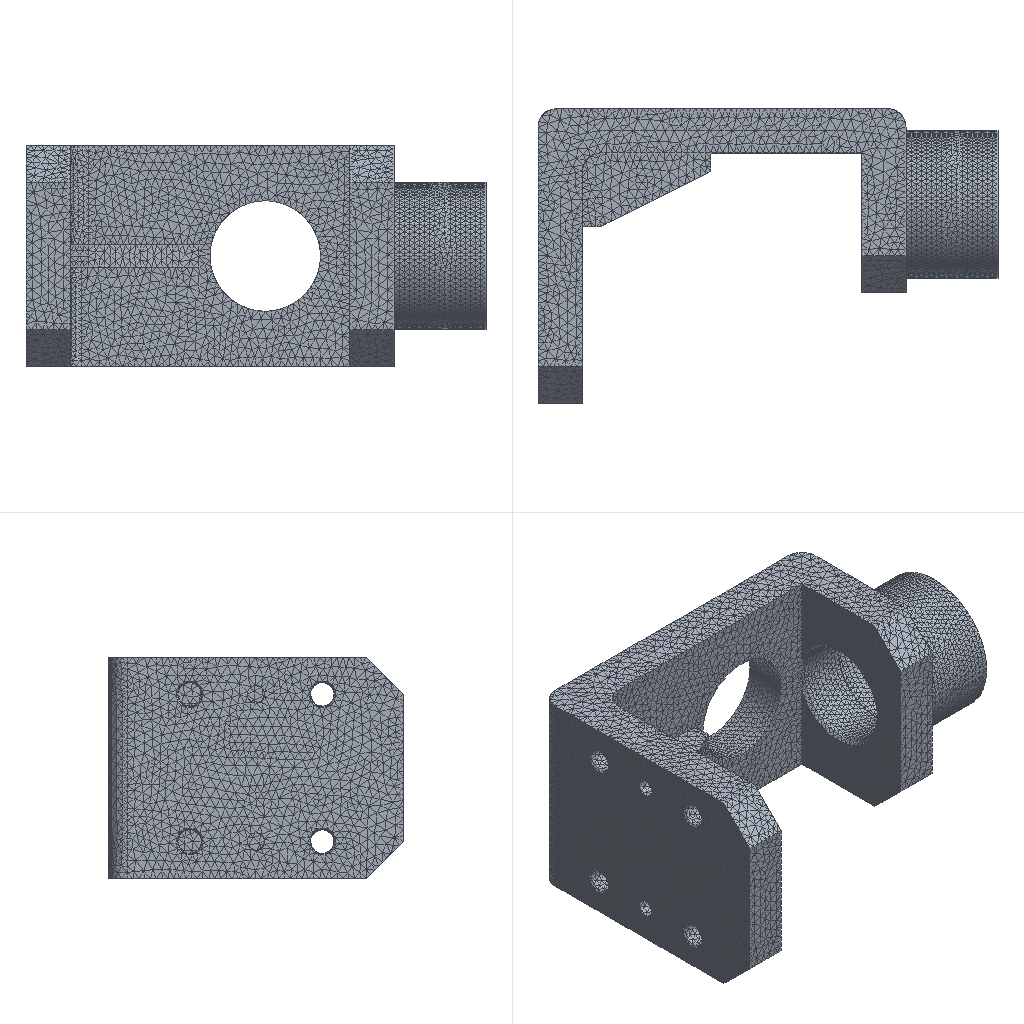Simulation study | ansys workbench
Set-up summary:
category,name,step,type,value,unit,region
solver,ansys_workbench
units,SI m-kg-s (Pa),,stated,"/units,MKS"
analysis,LS1,,static
load_step,LS1,LS1,static,nsubst=1; time=1
mesh,nodes,,,109969
mesh,elements,,,66278
element_type,SOLID187,,,66150
element_type,CONTA174,,,128
material,Structural Steel,,E,2e+11,Pa
material,Structural Steel,,nu,0.3
material,Structural Steel,,density,7850,kg m^-3
material,Structural Steel,,conductivity,60.5,W m^-1 C^-1
material,Structural Steel,,specific_heat,434,J kg^-1 C^-1
material,Structural Steel,,cte,1.2e-05,C^-1
material,Structural Steel,,permeability,10000
material,Structural Steel,,resistivity,1.7e-07,kg m^3 A^-2 s^-3
load,,LS1,moment,"5000 [dir=(1, 0, 0) n=3]",,all
bc,Fixed Supports,model,fixed,[dofs=ALL],,_FIXEDSU
contact,contact 1,,bonded (always),element=CONTA174
named_set,_FIXEDSU,,node,3748
Ansys APDL input file, long lists of numbers shortened:
/batch
/config,noeldb,1     ! force off writing results to database
*get,_wallstrt,active,,time,wall
! ANSYS input file written by Workbench version 2024 R1
! File used for geometry attach:
/title,wbnew--____ (A5)
! ****** Begin Custom Load Command Snippet ******
/COM, ACT Extensions:
/COM,     LSDYNA, 2024.1
/COM,/COM,     ANSYSMotion, 2024.1
/COM,
! ****** End   Custom Load Command Snippet ******
*DIM,_wb_ProjectScratch_dir,string,248
_wb_ProjectScratch_dir(1) = ''
*DIM,_wb_SolverFiles_dir,string,248
_wb_SolverFiles_dir(1) = ''
*DIM,_wb_userfiles_dir,string,248
_wb_userfiles_dir(1) = ''
/com,--- Data in consistent MKS units. See Solving Units in the help system for more information.
/units,MKS
/nopr
/wb,file,start              !  signify a WB generated input file
/prep7
! Turn off shape checking because checks already performed inside WB mesher.
! See help system for more information.
SHPP,OFF,,NOWARN
/nolist
etcon,set             ! allow ANSYS to choose best KEYOP's for 180x elements, resets any applicable keyopt to MAPDL defaults
/com,*********** Nodes for the whole assembly ***********
nblock,3,,120964
(1i9,3e20.9e3)
        1     1.030000000E-01     1.400000000E-02     1.750000000E-02
! (109967 more lines like these left out)
-1
/com,*********** Nodes for all Remote Points ***********
nblock,3
(1i9,3e20.9e3)
   109969     1.030000000E-01     1.401560474E-02     6.515581560E-07
-1
/wb,elem,start            !  set before creation of elements
/com,*********** Elements for Body 1 "2022" ***********
et,1,187
eblock,19,solid,,66150
(19i9)
        1        1        1        1        0        0        0        0       10        0        1     9118    16267    16605    16559    71457   109885    71459    71458
! (132299 more lines like these left out)
-1
/wb,elem,end               !  done creating elements
/com,*********** Send User Defined Coordinate System(s) ***********
csys,0
toffst,273.15,  ! Temperature offset from absolute zero
/com,*********** Set Reference Temperature ***********
tref,22.
/wb,mat,start              !  starting to send materials
/com,*********** Send Materials ***********
Temperature = 'TEMP' ! Temperature
MP,DENS,1,7850,	! kg m^-3
MP,ALPX,1,1.2e-05,	! C^-1
MP,C,1,434,	! J kg^-1 C^-1
MP,KXX,1,60.5,	! W m^-1 C^-1
MP,RSVX,1,1.7e-07,	! kg m^3 A^-2 s^-3
MP,EX,1,200000000000,	! Pa
MP,NUXY,1,0.3,
MP,MURX,1,10000,
/wb,mat,end                !  done sending materials
!************************* Model Summary ********************
!2022,	ç»æé¢,	matid,	1
!************************* End Model Summary ********************
! get the diagonal of the bounding box. Needed later for other things
*get,_xmin,node,,mnloc,x
*get,_ymin,node,,mnloc,y
*get,_zmin,node,,mnloc,z
*get,_xmax,node,,mxloc,x
*get,_ymax,node,,mxloc,y
*get,_zmax,node,,mxloc,z
_ASMDIAG=(_xmax-_xmin)*(_xmax-_xmin)+(_ymax-_ymin)*(_ymax-_ymin)+(_zmax-_zmin)*(_zmax-_zmin)
_ASMDIAG=SQRT(_ASMDIAG)
/wb,contact,start          !  starting to send contact
/wb,contact,end            !  done creating contacts
/golist
/wb,load,start             !  starting to send loads
/com,*********** Fixed Supports ***********
CMBLOCK,_FIXEDSU,NODE,     3748
(8i10)
       657       658       659       660       661       662       663       664
! (468 more lines like these left out)
cmsel,s,_FIXEDSU
d,all,all
nsel,all
/com,*********** Create Remote Point "ÄÚ²¿Ô¶³Ìµã" ***********
! -------- Remote Point Used by "Á¦¾Ø" --------
*set,tid,3
*set,cid,2
et,cid,174
et,tid,170
keyo,tid,2,1               ! Don't fix the pilot node
keyo,tid,4,111111
keyo,cid,12,5              ! Bonded Contact
keyo,cid,4,1               ! Deformable RBE3 style load
keyo,cid,2,2               ! MPC style contact
eblock,10,,,128
(15i9)
    87346        2        2        2        0       20     1799       21       21    16836    16846       21    16834
! (127 more lines like these left out)
-1
*set,_npilot,109969
_npilot33=_npilot
type,tid
mat ,cid
real,cid
tshape,pilo
en,87474,_npilot
tshape
/com,*********** Construct Moment Using Remote Attachment ***********
/gst,on,on
fini
*get,_numnode,node,0,count
*get,_numelem,elem,0,count
*get, _MAXELEMNUM, elem, 0, NUM, MAX
*get, _MAXNODENUM, node, 0, NUM, MAX
*get, _MAXELEMTYPE, etyp, 0, NUM, MAX
*get, _MAXREALCONST, rcon, 0, NUM, MAX
/go
/wb,load,end               !  done creating loads
/com,--- Number of total nodes = %_numnode%
/com,--- Number of contact elements = 128
/com,--- Number of spring elements = 0
/com,--- Number of bearing elements = 0
/com,--- Number of solid elements = 66150
/com,--- Number of condensed parts = 0
/com,--- Number of total elements = %_numelem%
*get,_wallbsol,active,,time,wall
/com,****************************************************************************
/com,*************************    SOLUTION       ********************************
/com,****************************************************************************
/solu
antype,0                   ! static analysis
_thickRatio=  1     ! Ratio of thick parts in the model
eqsl,pcg,1e-8,,,,,,1
cntr,print,1               ! print out contact info and also make no initial contact an error
cncheck,dmp		!	Enable program controlled contact splitting for distributed memory parallel run
dmpoption,emat,no             ! Don't combine emat file for DANSYS
dmpoption,esav,no             ! Don't combine esav file for DANSYS
nldiag,cont,iter           ! print out contact info each equilibrium iteration
rescontrol,,none                 ! Do not keep any restart files
/com,****************************************************
/com,******************* SOLVE FOR LS 1 OF 1 ****************
nsel,s,node,,109969
f,all,mx,5000.
f,all,my,0.
f,all,mz,0.
nsel,all
/nopr
/gopr
nsub,1,1,1
time,1.
outres,erase
outres,all,none
outres,nsol,all,
outres,rsol,all
outres,eangl,all
outres,etmp,all
outres,veng,all
outres,strs,all,
outres,epel,all,
outres,eppl,all,
outres,cont,all,
! *********** WB SOLVE COMMAND ***********
! check interactive state
*get,ANSINTER_,active,,int
*if,ANSINTER_,ne,0,then
/eof
*endif
solve
/com *************** Write FE CONNECTORS *********
CEWRITE,file,ce,,INTE
/com,****************************************************
/com,*************** FINISHED SOLVE FOR LS 1 *************
*get,_wallasol,active,,time,wall
/nopr
*get,_numnode,node,0,count
*get,_numelem,elem,0,count
*get, _MAXELEMNUM, elem, 0, NUM, MAX
*get, _MAXNODENUM, node, 0, NUM, MAX,,,INTERNAL
*get, _MAXELEMTYPE, etyp, 0, NUM, MAX
*get, _MAXREALCONST, rcon, 0, NUM, MAX
*get,_NSOLTHREADS,active,0,ntfs
*get,_NSOLPROCESSES,active,0,npfs
/gopr
*get,_PCGITER,active,,solu,cgiter
/post1
xmlo,ENCODING,ISO-8859-1
xmlo,parm
/xml,parm,xml
fini
/gopr
*get,_walldone,active,,time,wall
_preptime=(_wallbsol-_wallstrt)*3600
_solvtime=(_wallasol-_wallbsol)*3600
_posttime=(_walldone-_wallasol)*3600
_totaltim=(_walldone-_wallstrt)*3600
*get,_dlbratio,active,0,solu,dlbr
*get,_combtime,active,0,solu,comb
*get,_ssmode,active,0,solu,ssmm
*get,_ndofs,active,0,solu,ndof
*get,_sol_end_time,active,0,set,time
*if,_sol_end_time,eq,1.,then
/fclean				!clean distributed files
*endif
/com,--- Total number of nodes = %_numnode%
/com,--- Total number of elements = %_numelem%
/com,--- Element load balance ratio = %_dlbratio%
/com,--- Time to combine distributed files = %_combtime%
/com,--- Sparse memory mode = %_ssmode%
/com,--- Number of DOF = %_ndofs%
/wb,file,end               ! done with WB generated input
Results summary:
result,analyses[0].index,,,1
result,analyses[0].system,,,SYS
result,analyses[0].deck,,,deck.dat
result,analyses[0].solve_status,,,completed
result,analyses[0].analysis_type,,,static
result,analyses[0].physics,,,mechanical
result,analyses[0].unit_system,,,"MKS: m, kg, N, s, V, A, degC"
result,analyses[0].n_sets,,,1
result,analyses[0].load_steps[0].set,set=1,,1
result,analyses[0].load_steps[0].time_or_freq,set=1,,1
result,analyses[0].load_steps[0].max_displacement_magnitude,set=1,,0.00943
result,analyses[0].load_steps[0].max_von_mises_nodal,set=1,,7.54065e+09
result,analyses[0].load_steps[0].reaction_force_sum_xyz[1],set=1,,-0.0001514
result,analyses[0].load_steps[0].reaction_force_sum_xyz[2],set=1,,0.0004688
result,analyses[0].load_steps[0].reaction_force_sum_xyz[3],set=1,,0.0004869
result,geometry_export[0][0],,,.step
result,geometry_export[0][1],,,ok
result,geometry_export[0][2],,,1